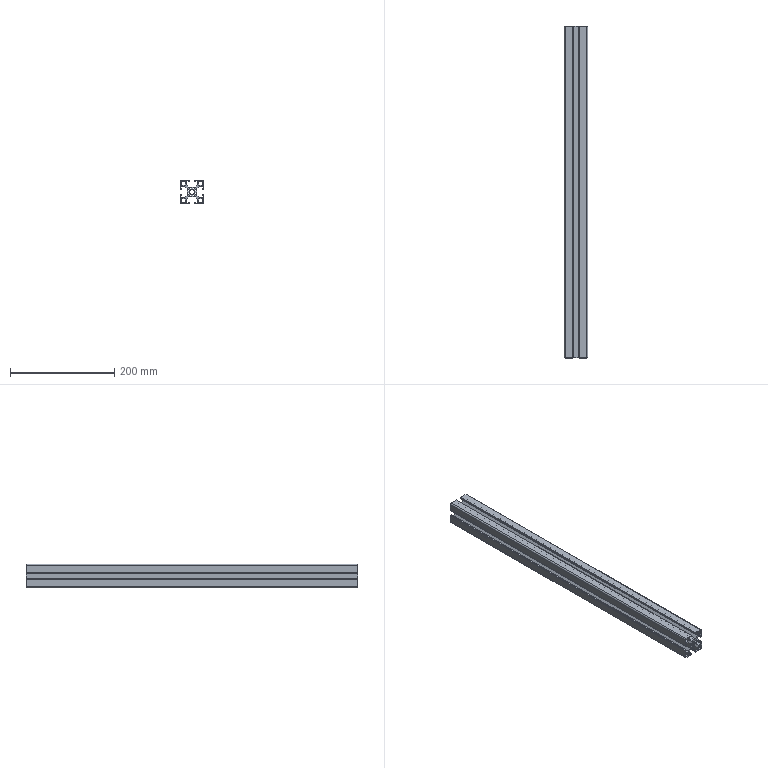Part | STEP file | 1 solid | 135 faces | box 45 x 636 x 45 mm | volume 440296 mm3 | plane 118 | cylinder 17 | commonest cylinder face diameters 10 x9 3 x4 5 x4